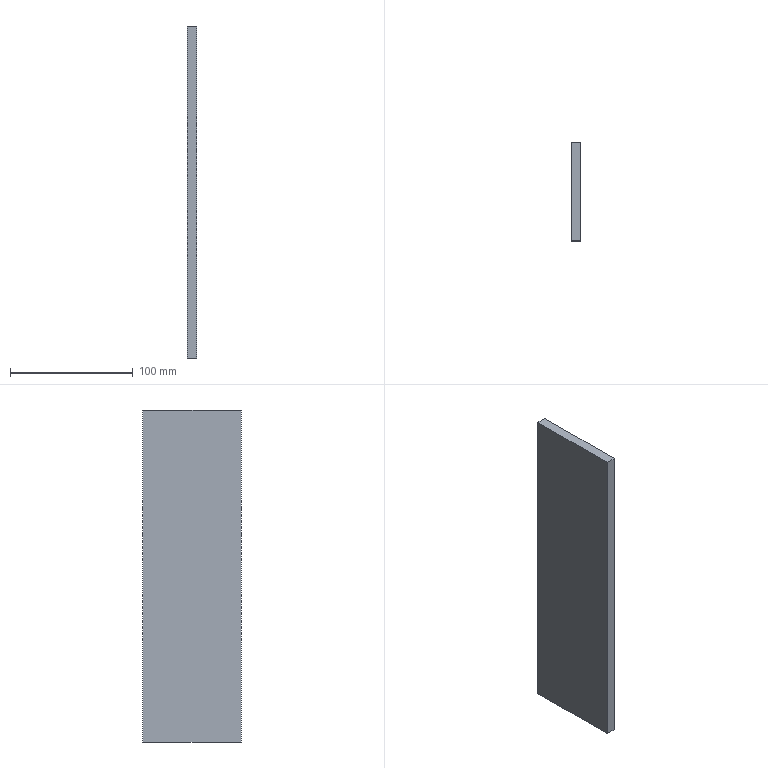Part | STEP file | X77-07103 | 1 solid | 6 faces | box 8 x 80 x 270 mm | volume 172800 mm3 | plane 6
STEP:
#1=CARTESIAN_POINT('',(-118.199,-80.,0.));
#2=VERTEX_POINT('',#1);
#3=CARTESIAN_POINT('',(-118.199,0.,0.));
#4=VERTEX_POINT('',#3);
#5=CARTESIAN_POINT('',(-118.199,0.,0.));
#6=DIRECTION('',(0.,1.,0.));
#7=VECTOR('',#6,1000.);
#8=LINE('',#5,#7);
#9=EDGE_CURVE('',#2,#4,#8,.T.);
#10=ORIENTED_EDGE('',*,*,#9,.T.);
#11=CARTESIAN_POINT('',(-118.199,0.,270.));
#12=VERTEX_POINT('',#11);
#13=CARTESIAN_POINT('',(-118.199,0.,270.));
#14=DIRECTION('',(0.,0.,-1.));
#15=VECTOR('',#14,1000.);
#16=LINE('',#13,#15);
#17=EDGE_CURVE('',#12,#4,#16,.T.);
#18=ORIENTED_EDGE('',*,*,#17,.F.);
#19=CARTESIAN_POINT('',(-118.199,-80.,270.));
#20=VERTEX_POINT('',#19);
#21=CARTESIAN_POINT('',(-118.199,0.,270.));
#22=DIRECTION('',(0.,1.,0.));
#23=VECTOR('',#22,1000.);
#24=LINE('',#21,#23);
#25=EDGE_CURVE('',#20,#12,#24,.T.);
#26=ORIENTED_EDGE('',*,*,#25,.F.);
#27=CARTESIAN_POINT('',(-118.199,-80.,270.));
#28=DIRECTION('',(0.,0.,-1.));
#29=VECTOR('',#28,1000.);
#30=LINE('',#27,#29);
#31=EDGE_CURVE('',#20,#2,#30,.T.);
#32=ORIENTED_EDGE('',*,*,#31,.T.);
#33=EDGE_LOOP('',(#10,#18,#26,#32));
#34=FACE_OUTER_BOUND('',#33,.T.);
#35=CARTESIAN_POINT('',(-118.199,0.,270.));
#36=DIRECTION('',(-1.,0.,0.));
#37=DIRECTION('',(0.,-1.,0.));
#38=AXIS2_PLACEMENT_3D('',#35,#36,#37);
#39=PLANE('',#38);
#40=ADVANCED_FACE('',(#34),#39,.F.);
#41=CARTESIAN_POINT('',(-126.199,0.,0.));
#42=VERTEX_POINT('',#41);
#43=CARTESIAN_POINT('',(-118.199,0.,0.));
#44=DIRECTION('',(-1.,0.,0.));
#45=VECTOR('',#44,1000.);
#46=LINE('',#43,#45);
#47=EDGE_CURVE('',#4,#42,#46,.T.);
#48=ORIENTED_EDGE('',*,*,#47,.T.);
#49=CARTESIAN_POINT('',(-126.199,0.,270.));
#50=VERTEX_POINT('',#49);
#51=CARTESIAN_POINT('',(-126.199,0.,270.));
#52=DIRECTION('',(0.,0.,-1.));
#53=VECTOR('',#52,1000.);
#54=LINE('',#51,#53);
#55=EDGE_CURVE('',#50,#42,#54,.T.);
#56=ORIENTED_EDGE('',*,*,#55,.F.);
#57=CARTESIAN_POINT('',(-118.199,0.,270.));
#58=DIRECTION('',(-1.,0.,0.));
#59=VECTOR('',#58,1000.);
#60=LINE('',#57,#59);
#61=EDGE_CURVE('',#12,#50,#60,.T.);
#62=ORIENTED_EDGE('',*,*,#61,.F.);
#63=ORIENTED_EDGE('',*,*,#17,.T.);
#64=EDGE_LOOP('',(#48,#56,#62,#63));
#65=FACE_OUTER_BOUND('',#64,.T.);
#66=CARTESIAN_POINT('',(-118.199,0.,270.));
#67=DIRECTION('',(0.,-1.,0.));
#68=DIRECTION('',(1.,0.,0.));
#69=AXIS2_PLACEMENT_3D('',#66,#67,#68);
#70=PLANE('',#69);
#71=ADVANCED_FACE('',(#65),#70,.F.);
#72=CARTESIAN_POINT('',(-126.199,-80.,0.));
#73=VERTEX_POINT('',#72);
#74=CARTESIAN_POINT('',(-126.199,0.,0.));
#75=DIRECTION('',(0.,-1.,0.));
#76=VECTOR('',#75,1000.);
#77=LINE('',#74,#76);
#78=EDGE_CURVE('',#42,#73,#77,.T.);
#79=ORIENTED_EDGE('',*,*,#78,.T.);
#80=CARTESIAN_POINT('',(-126.199,-80.,270.));
#81=VERTEX_POINT('',#80);
#82=CARTESIAN_POINT('',(-126.199,-80.,270.));
#83=DIRECTION('',(0.,0.,-1.));
#84=VECTOR('',#83,1000.);
#85=LINE('',#82,#84);
#86=EDGE_CURVE('',#81,#73,#85,.T.);
#87=ORIENTED_EDGE('',*,*,#86,.F.);
#88=CARTESIAN_POINT('',(-126.199,0.,270.));
#89=DIRECTION('',(0.,-1.,0.));
#90=VECTOR('',#89,1000.);
#91=LINE('',#88,#90);
#92=EDGE_CURVE('',#50,#81,#91,.T.);
#93=ORIENTED_EDGE('',*,*,#92,.F.);
#94=ORIENTED_EDGE('',*,*,#55,.T.);
#95=EDGE_LOOP('',(#79,#87,#93,#94));
#96=FACE_OUTER_BOUND('',#95,.T.);
#97=CARTESIAN_POINT('',(-126.199,0.,270.));
#98=DIRECTION('',(1.,0.,0.));
#99=DIRECTION('',(0.,1.,0.));
#100=AXIS2_PLACEMENT_3D('',#97,#98,#99);
#101=PLANE('',#100);
#102=ADVANCED_FACE('',(#96),#101,.F.);
#103=CARTESIAN_POINT('',(-118.199,-80.,0.));
#104=DIRECTION('',(1.,0.,0.));
#105=VECTOR('',#104,1000.);
#106=LINE('',#103,#105);
#107=EDGE_CURVE('',#73,#2,#106,.T.);
#108=ORIENTED_EDGE('',*,*,#107,.T.);
#109=ORIENTED_EDGE('',*,*,#31,.F.);
#110=CARTESIAN_POINT('',(-118.199,-80.,270.));
#111=DIRECTION('',(1.,0.,0.));
#112=VECTOR('',#111,1000.);
#113=LINE('',#110,#112);
#114=EDGE_CURVE('',#81,#20,#113,.T.);
#115=ORIENTED_EDGE('',*,*,#114,.F.);
#116=ORIENTED_EDGE('',*,*,#86,.T.);
#117=EDGE_LOOP('',(#108,#109,#115,#116));
#118=FACE_OUTER_BOUND('',#117,.T.);
#119=CARTESIAN_POINT('',(-118.199,-80.,270.));
#120=DIRECTION('',(0.,1.,0.));
#121=DIRECTION('',(0.,0.,1.));
#122=AXIS2_PLACEMENT_3D('',#119,#120,#121);
#123=PLANE('',#122);
#124=ADVANCED_FACE('',(#118),#123,.F.);
#125=ORIENTED_EDGE('',*,*,#25,.T.);
#126=ORIENTED_EDGE('',*,*,#61,.T.);
#127=ORIENTED_EDGE('',*,*,#92,.T.);
#128=ORIENTED_EDGE('',*,*,#114,.T.);
#129=EDGE_LOOP('',(#125,#126,#127,#128));
#130=FACE_OUTER_BOUND('',#129,.T.);
#131=CARTESIAN_POINT('',(-118.199,-80.,270.));
#132=DIRECTION('',(0.,0.,-1.));
#133=DIRECTION('',(-1.,0.,0.));
#134=AXIS2_PLACEMENT_3D('',#131,#132,#133);
#135=PLANE('',#134);
#136=ADVANCED_FACE('',(#130),#135,.F.);
#137=ORIENTED_EDGE('',*,*,#9,.F.);
#138=ORIENTED_EDGE('',*,*,#107,.F.);
#139=ORIENTED_EDGE('',*,*,#78,.F.);
#140=ORIENTED_EDGE('',*,*,#47,.F.);
#141=EDGE_LOOP('',(#137,#138,#139,#140));
#142=FACE_OUTER_BOUND('',#141,.T.);
#143=CARTESIAN_POINT('',(-118.199,-80.,0.));
#144=DIRECTION('',(0.,0.,-1.));
#145=DIRECTION('',(-1.,0.,0.));
#146=AXIS2_PLACEMENT_3D('',#143,#144,#145);
#147=PLANE('',#146);
#148=ADVANCED_FACE('',(#142),#147,.T.);
#149=CLOSED_SHELL('',(#40,#71,#102,#124,#136,#148));
#150=MANIFOLD_SOLID_BREP('',#149);
#151=CARTESIAN_POINT('',(0.,0.,0.));
#152=DIRECTION('',(0.,0.,1.));
#153=DIRECTION('',(1.,0.,0.));
#154=AXIS2_PLACEMENT_3D('',#151,#152,#153);
#155=(LENGTH_UNIT()NAMED_UNIT(*)SI_UNIT(.MILLI.,.METRE.));
#156=UNCERTAINTY_MEASURE_WITH_UNIT(LENGTH_MEASURE(0.00001),#155,'','');
#157=(NAMED_UNIT(*)PLANE_ANGLE_UNIT()SI_UNIT($,.RADIAN.));
#158=(NAMED_UNIT(*)SI_UNIT($,.STERADIAN.)SOLID_ANGLE_UNIT());
#159=(GEOMETRIC_REPRESENTATION_CONTEXT(3)GLOBAL_UNCERTAINTY_ASSIGNED_CONTEXT((#156))GLOBAL_UNIT_ASSIGNED_CONTEXT((#155,#157,#158))REPRESENTATION_CONTEXT('',''));
#160=ADVANCED_BREP_SHAPE_REPRESENTATION('',(#150,#154),#159);